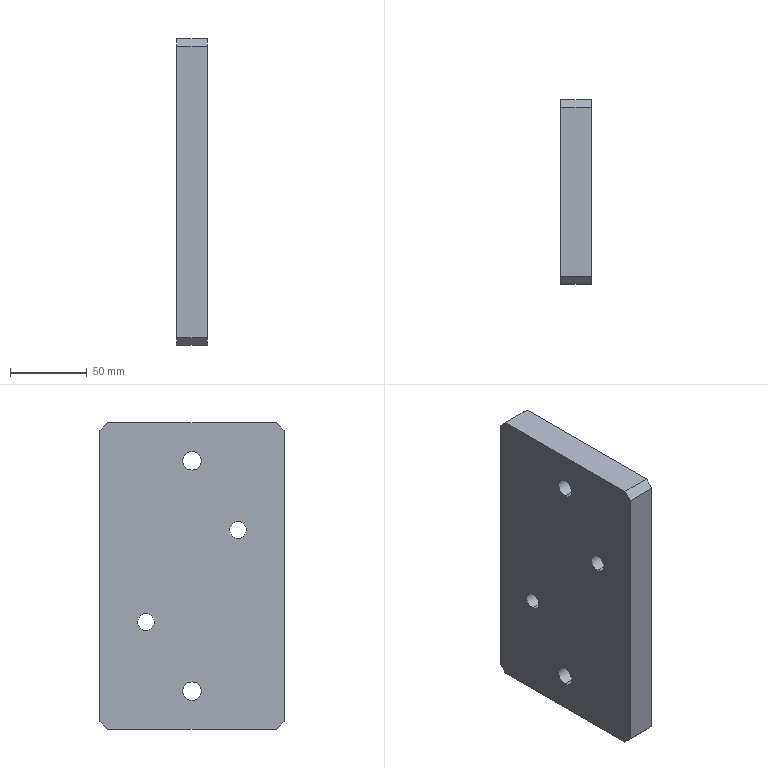Part | SolidWorks | features HoleWzd 2, Chamfer 1, Extrusion 1 | 1 solid | 24 faces | box 20 x 120 x 200 mm | volume 467167 mm3 | cylinder 12 | plane 12 | commonest cylinder face diameters 11 x4 12 x4 18 x4
STEP:
#1=CARTESIAN_POINT('',(0.,0.,81.));
#2=VERTEX_POINT('',#1);
#3=CARTESIAN_POINT('',(0.,0.,69.));
#4=VERTEX_POINT('',#3);
#5=CARTESIAN_POINT('',(0.,0.,75.));
#6=DIRECTION('',(1.,0.,0.));
#7=DIRECTION('',(0.,0.,-1.));
#8=AXIS2_PLACEMENT_3D('',#5,#6,#7);
#9=CIRCLE('',#8,6.);
#10=EDGE_CURVE('',#2,#4,#9,.T.);
#11=ORIENTED_EDGE('',*,*,#10,.F.);
#12=CARTESIAN_POINT('',(20.,0.,81.));
#13=VERTEX_POINT('',#12);
#14=CARTESIAN_POINT('',(20.,0.,81.));
#15=DIRECTION('',(1.,0.,0.));
#16=VECTOR('',#15,1000.);
#17=LINE('',#14,#16);
#18=EDGE_CURVE('',#2,#13,#17,.T.);
#19=ORIENTED_EDGE('',*,*,#18,.T.);
#20=CARTESIAN_POINT('',(20.,0.,69.));
#21=VERTEX_POINT('',#20);
#22=CARTESIAN_POINT('',(20.,0.,75.));
#23=DIRECTION('',(1.,0.,0.));
#24=DIRECTION('',(0.,0.,-1.));
#25=AXIS2_PLACEMENT_3D('',#22,#23,#24);
#26=CIRCLE('',#25,6.);
#27=EDGE_CURVE('',#13,#21,#26,.T.);
#28=ORIENTED_EDGE('',*,*,#27,.T.);
#29=CARTESIAN_POINT('',(20.,0.,69.));
#30=DIRECTION('',(1.,0.,0.));
#31=VECTOR('',#30,1000.);
#32=LINE('',#29,#31);
#33=EDGE_CURVE('',#4,#21,#32,.T.);
#34=ORIENTED_EDGE('',*,*,#33,.F.);
#35=EDGE_LOOP('',(#11,#19,#28,#34));
#36=FACE_OUTER_BOUND('',#35,.T.);
#37=CARTESIAN_POINT('',(20.,0.,75.));
#38=DIRECTION('',(1.,0.,0.));
#39=DIRECTION('',(0.,0.,-1.));
#40=AXIS2_PLACEMENT_3D('',#37,#38,#39);
#41=CYLINDRICAL_SURFACE('',#40,6.);
#42=ADVANCED_FACE('',(#36),#41,.F.);
#43=CARTESIAN_POINT('',(0.,0.,-69.));
#44=VERTEX_POINT('',#43);
#45=CARTESIAN_POINT('',(0.,0.,-81.));
#46=VERTEX_POINT('',#45);
#47=CARTESIAN_POINT('',(0.,0.,-75.));
#48=DIRECTION('',(1.,0.,0.));
#49=DIRECTION('',(0.,0.,-1.));
#50=AXIS2_PLACEMENT_3D('',#47,#48,#49);
#51=CIRCLE('',#50,6.);
#52=EDGE_CURVE('',#44,#46,#51,.T.);
#53=ORIENTED_EDGE('',*,*,#52,.F.);
#54=CARTESIAN_POINT('',(20.,0.,-69.));
#55=VERTEX_POINT('',#54);
#56=CARTESIAN_POINT('',(20.,0.,-69.));
#57=DIRECTION('',(1.,0.,0.));
#58=VECTOR('',#57,1000.);
#59=LINE('',#56,#58);
#60=EDGE_CURVE('',#44,#55,#59,.T.);
#61=ORIENTED_EDGE('',*,*,#60,.T.);
#62=CARTESIAN_POINT('',(20.,0.,-81.));
#63=VERTEX_POINT('',#62);
#64=CARTESIAN_POINT('',(20.,0.,-75.));
#65=DIRECTION('',(1.,0.,0.));
#66=DIRECTION('',(0.,0.,-1.));
#67=AXIS2_PLACEMENT_3D('',#64,#65,#66);
#68=CIRCLE('',#67,6.);
#69=EDGE_CURVE('',#55,#63,#68,.T.);
#70=ORIENTED_EDGE('',*,*,#69,.T.);
#71=CARTESIAN_POINT('',(20.,0.,-81.));
#72=DIRECTION('',(1.,0.,0.));
#73=VECTOR('',#72,1000.);
#74=LINE('',#71,#73);
#75=EDGE_CURVE('',#46,#63,#74,.T.);
#76=ORIENTED_EDGE('',*,*,#75,.F.);
#77=EDGE_LOOP('',(#53,#61,#70,#76));
#78=FACE_OUTER_BOUND('',#77,.T.);
#79=CARTESIAN_POINT('',(20.,0.,-75.));
#80=DIRECTION('',(1.,0.,0.));
#81=DIRECTION('',(0.,0.,-1.));
#82=AXIS2_PLACEMENT_3D('',#79,#80,#81);
#83=CYLINDRICAL_SURFACE('',#82,6.);
#84=ADVANCED_FACE('',(#78),#83,.F.);
#85=CARTESIAN_POINT('',(9.,30.,-21.));
#86=VERTEX_POINT('',#85);
#87=CARTESIAN_POINT('',(9.,30.,-39.));
#88=VERTEX_POINT('',#87);
#89=CARTESIAN_POINT('',(9.,30.,-30.));
#90=DIRECTION('',(1.,0.,0.));
#91=DIRECTION('',(0.,0.,-1.));
#92=AXIS2_PLACEMENT_3D('',#89,#90,#91);
#93=CIRCLE('',#92,9.);
#94=EDGE_CURVE('',#86,#88,#93,.T.);
#95=ORIENTED_EDGE('',*,*,#94,.F.);
#96=CARTESIAN_POINT('',(20.,30.,-21.));
#97=VERTEX_POINT('',#96);
#98=CARTESIAN_POINT('',(20.,30.,-21.));
#99=DIRECTION('',(1.,0.,0.));
#100=VECTOR('',#99,1000.);
#101=LINE('',#98,#100);
#102=EDGE_CURVE('',#86,#97,#101,.T.);
#103=ORIENTED_EDGE('',*,*,#102,.T.);
#104=CARTESIAN_POINT('',(20.,30.,-39.));
#105=VERTEX_POINT('',#104);
#106=CARTESIAN_POINT('',(20.,30.,-30.));
#107=DIRECTION('',(1.,0.,0.));
#108=DIRECTION('',(0.,0.,-1.));
#109=AXIS2_PLACEMENT_3D('',#106,#107,#108);
#110=CIRCLE('',#109,9.);
#111=EDGE_CURVE('',#97,#105,#110,.T.);
#112=ORIENTED_EDGE('',*,*,#111,.T.);
#113=CARTESIAN_POINT('',(20.,30.,-39.));
#114=DIRECTION('',(1.,0.,0.));
#115=VECTOR('',#114,1000.);
#116=LINE('',#113,#115);
#117=EDGE_CURVE('',#88,#105,#116,.T.);
#118=ORIENTED_EDGE('',*,*,#117,.F.);
#119=EDGE_LOOP('',(#95,#103,#112,#118));
#120=FACE_OUTER_BOUND('',#119,.T.);
#121=CARTESIAN_POINT('',(20.,30.,-30.));
#122=DIRECTION('',(1.,0.,0.));
#123=DIRECTION('',(0.,0.,-1.));
#124=AXIS2_PLACEMENT_3D('',#121,#122,#123);
#125=CYLINDRICAL_SURFACE('',#124,9.);
#126=ADVANCED_FACE('',(#120),#125,.F.);
#127=CARTESIAN_POINT('',(0.,30.,-24.5));
#128=VERTEX_POINT('',#127);
#129=CARTESIAN_POINT('',(0.,30.,-35.5));
#130=VERTEX_POINT('',#129);
#131=CARTESIAN_POINT('',(0.,30.,-30.));
#132=DIRECTION('',(1.,0.,0.));
#133=DIRECTION('',(0.,0.,-1.));
#134=AXIS2_PLACEMENT_3D('',#131,#132,#133);
#135=CIRCLE('',#134,5.5);
#136=EDGE_CURVE('',#128,#130,#135,.T.);
#137=ORIENTED_EDGE('',*,*,#136,.F.);
#138=CARTESIAN_POINT('',(9.,30.,-24.5));
#139=VERTEX_POINT('',#138);
#140=CARTESIAN_POINT('',(20.,30.,-24.5));
#141=DIRECTION('',(1.,0.,0.));
#142=VECTOR('',#141,1000.);
#143=LINE('',#140,#142);
#144=EDGE_CURVE('',#128,#139,#143,.T.);
#145=ORIENTED_EDGE('',*,*,#144,.T.);
#146=CARTESIAN_POINT('',(9.,30.,-35.5));
#147=VERTEX_POINT('',#146);
#148=CARTESIAN_POINT('',(9.,30.,-30.));
#149=DIRECTION('',(1.,0.,0.));
#150=DIRECTION('',(0.,0.,-1.));
#151=AXIS2_PLACEMENT_3D('',#148,#149,#150);
#152=CIRCLE('',#151,5.5);
#153=EDGE_CURVE('',#139,#147,#152,.T.);
#154=ORIENTED_EDGE('',*,*,#153,.T.);
#155=CARTESIAN_POINT('',(20.,30.,-35.5));
#156=DIRECTION('',(1.,0.,0.));
#157=VECTOR('',#156,1000.);
#158=LINE('',#155,#157);
#159=EDGE_CURVE('',#130,#147,#158,.T.);
#160=ORIENTED_EDGE('',*,*,#159,.F.);
#161=EDGE_LOOP('',(#137,#145,#154,#160));
#162=FACE_OUTER_BOUND('',#161,.T.);
#163=CARTESIAN_POINT('',(20.,30.,-30.));
#164=DIRECTION('',(1.,0.,0.));
#165=DIRECTION('',(0.,0.,-1.));
#166=AXIS2_PLACEMENT_3D('',#163,#164,#165);
#167=CYLINDRICAL_SURFACE('',#166,5.5);
#168=ADVANCED_FACE('',(#162),#167,.F.);
#169=CARTESIAN_POINT('',(9.,-30.,39.));
#170=VERTEX_POINT('',#169);
#171=CARTESIAN_POINT('',(9.,-30.,21.));
#172=VERTEX_POINT('',#171);
#173=CARTESIAN_POINT('',(9.,-30.,30.));
#174=DIRECTION('',(1.,0.,0.));
#175=DIRECTION('',(0.,0.,-1.));
#176=AXIS2_PLACEMENT_3D('',#173,#174,#175);
#177=CIRCLE('',#176,9.);
#178=EDGE_CURVE('',#170,#172,#177,.T.);
#179=ORIENTED_EDGE('',*,*,#178,.F.);
#180=CARTESIAN_POINT('',(20.,-30.,39.));
#181=VERTEX_POINT('',#180);
#182=CARTESIAN_POINT('',(20.,-30.,39.));
#183=DIRECTION('',(1.,0.,0.));
#184=VECTOR('',#183,1000.);
#185=LINE('',#182,#184);
#186=EDGE_CURVE('',#170,#181,#185,.T.);
#187=ORIENTED_EDGE('',*,*,#186,.T.);
#188=CARTESIAN_POINT('',(20.,-30.,21.));
#189=VERTEX_POINT('',#188);
#190=CARTESIAN_POINT('',(20.,-30.,30.));
#191=DIRECTION('',(1.,0.,0.));
#192=DIRECTION('',(0.,0.,-1.));
#193=AXIS2_PLACEMENT_3D('',#190,#191,#192);
#194=CIRCLE('',#193,9.);
#195=EDGE_CURVE('',#181,#189,#194,.T.);
#196=ORIENTED_EDGE('',*,*,#195,.T.);
#197=CARTESIAN_POINT('',(20.,-30.,21.));
#198=DIRECTION('',(1.,0.,0.));
#199=VECTOR('',#198,1000.);
#200=LINE('',#197,#199);
#201=EDGE_CURVE('',#172,#189,#200,.T.);
#202=ORIENTED_EDGE('',*,*,#201,.F.);
#203=EDGE_LOOP('',(#179,#187,#196,#202));
#204=FACE_OUTER_BOUND('',#203,.T.);
#205=CARTESIAN_POINT('',(20.,-30.,30.));
#206=DIRECTION('',(1.,0.,0.));
#207=DIRECTION('',(0.,0.,-1.));
#208=AXIS2_PLACEMENT_3D('',#205,#206,#207);
#209=CYLINDRICAL_SURFACE('',#208,9.);
#210=ADVANCED_FACE('',(#204),#209,.F.);
#211=CARTESIAN_POINT('',(0.,-30.,35.5));
#212=VERTEX_POINT('',#211);
#213=CARTESIAN_POINT('',(0.,-30.,24.5));
#214=VERTEX_POINT('',#213);
#215=CARTESIAN_POINT('',(0.,-30.,30.));
#216=DIRECTION('',(1.,0.,0.));
#217=DIRECTION('',(0.,0.,-1.));
#218=AXIS2_PLACEMENT_3D('',#215,#216,#217);
#219=CIRCLE('',#218,5.5);
#220=EDGE_CURVE('',#212,#214,#219,.T.);
#221=ORIENTED_EDGE('',*,*,#220,.F.);
#222=CARTESIAN_POINT('',(9.,-30.,35.5));
#223=VERTEX_POINT('',#222);
#224=CARTESIAN_POINT('',(20.,-30.,35.5));
#225=DIRECTION('',(1.,0.,0.));
#226=VECTOR('',#225,1000.);
#227=LINE('',#224,#226);
#228=EDGE_CURVE('',#212,#223,#227,.T.);
#229=ORIENTED_EDGE('',*,*,#228,.T.);
#230=CARTESIAN_POINT('',(9.,-30.,24.5));
#231=VERTEX_POINT('',#230);
#232=CARTESIAN_POINT('',(9.,-30.,30.));
#233=DIRECTION('',(1.,0.,0.));
#234=DIRECTION('',(0.,0.,-1.));
#235=AXIS2_PLACEMENT_3D('',#232,#233,#234);
#236=CIRCLE('',#235,5.5);
#237=EDGE_CURVE('',#223,#231,#236,.T.);
#238=ORIENTED_EDGE('',*,*,#237,.T.);
#239=CARTESIAN_POINT('',(20.,-30.,24.5));
#240=DIRECTION('',(1.,0.,0.));
#241=VECTOR('',#240,1000.);
#242=LINE('',#239,#241);
#243=EDGE_CURVE('',#214,#231,#242,.T.);
#244=ORIENTED_EDGE('',*,*,#243,.F.);
#245=EDGE_LOOP('',(#221,#229,#238,#244));
#246=FACE_OUTER_BOUND('',#245,.T.);
#247=CARTESIAN_POINT('',(20.,-30.,30.));
#248=DIRECTION('',(1.,0.,0.));
#249=DIRECTION('',(0.,0.,-1.));
#250=AXIS2_PLACEMENT_3D('',#247,#248,#249);
#251=CYLINDRICAL_SURFACE('',#250,5.5);
#252=ADVANCED_FACE('',(#246),#251,.F.);
#253=CARTESIAN_POINT('',(0.,-55.,-100.));
#254=VERTEX_POINT('',#253);
#255=CARTESIAN_POINT('',(0.,55.,-100.));
#256=VERTEX_POINT('',#255);
#257=CARTESIAN_POINT('',(0.,60.,-100.));
#258=DIRECTION('',(0.,1.,0.));
#259=VECTOR('',#258,1000.);
#260=LINE('',#257,#259);
#261=EDGE_CURVE('',#254,#256,#260,.T.);
#262=ORIENTED_EDGE('',*,*,#261,.T.);
#263=CARTESIAN_POINT('',(20.,55.,-100.));
#264=VERTEX_POINT('',#263);
#265=CARTESIAN_POINT('',(20.,55.,-100.));
#266=DIRECTION('',(1.,0.,0.));
#267=VECTOR('',#266,1000.);
#268=LINE('',#265,#267);
#269=EDGE_CURVE('',#256,#264,#268,.T.);
#270=ORIENTED_EDGE('',*,*,#269,.T.);
#271=CARTESIAN_POINT('',(20.,-55.,-100.));
#272=VERTEX_POINT('',#271);
#273=CARTESIAN_POINT('',(20.,60.,-100.));
#274=DIRECTION('',(0.,1.,0.));
#275=VECTOR('',#274,1000.);
#276=LINE('',#273,#275);
#277=EDGE_CURVE('',#272,#264,#276,.T.);
#278=ORIENTED_EDGE('',*,*,#277,.F.);
#279=CARTESIAN_POINT('',(20.,-55.,-100.));
#280=DIRECTION('',(-1.,0.,0.));
#281=VECTOR('',#280,1000.);
#282=LINE('',#279,#281);
#283=EDGE_CURVE('',#272,#254,#282,.T.);
#284=ORIENTED_EDGE('',*,*,#283,.T.);
#285=EDGE_LOOP('',(#262,#270,#278,#284));
#286=FACE_OUTER_BOUND('',#285,.T.);
#287=CARTESIAN_POINT('',(20.,60.,-100.));
#288=DIRECTION('',(0.,0.,1.));
#289=DIRECTION('',(0.,-1.,0.));
#290=AXIS2_PLACEMENT_3D('',#287,#288,#289);
#291=PLANE('',#290);
#292=ADVANCED_FACE('',(#286),#291,.F.);
#293=CARTESIAN_POINT('',(0.,60.,-95.));
#294=VERTEX_POINT('',#293);
#295=CARTESIAN_POINT('',(0.,60.,95.));
#296=VERTEX_POINT('',#295);
#297=CARTESIAN_POINT('',(0.,60.,100.));
#298=DIRECTION('',(0.,0.,1.));
#299=VECTOR('',#298,1000.);
#300=LINE('',#297,#299);
#301=EDGE_CURVE('',#294,#296,#300,.T.);
#302=ORIENTED_EDGE('',*,*,#301,.T.);
#303=CARTESIAN_POINT('',(20.,60.,95.));
#304=VERTEX_POINT('',#303);
#305=CARTESIAN_POINT('',(20.,60.,95.));
#306=DIRECTION('',(1.,0.,0.));
#307=VECTOR('',#306,1000.);
#308=LINE('',#305,#307);
#309=EDGE_CURVE('',#296,#304,#308,.T.);
#310=ORIENTED_EDGE('',*,*,#309,.T.);
#311=CARTESIAN_POINT('',(20.,60.,-95.));
#312=VERTEX_POINT('',#311);
#313=CARTESIAN_POINT('',(20.,60.,100.));
#314=DIRECTION('',(0.,0.,1.));
#315=VECTOR('',#314,1000.);
#316=LINE('',#313,#315);
#317=EDGE_CURVE('',#312,#304,#316,.T.);
#318=ORIENTED_EDGE('',*,*,#317,.F.);
#319=CARTESIAN_POINT('',(20.,60.,-95.));
#320=DIRECTION('',(-1.,0.,0.));
#321=VECTOR('',#320,1000.);
#322=LINE('',#319,#321);
#323=EDGE_CURVE('',#312,#294,#322,.T.);
#324=ORIENTED_EDGE('',*,*,#323,.T.);
#325=EDGE_LOOP('',(#302,#310,#318,#324));
#326=FACE_OUTER_BOUND('',#325,.T.);
#327=CARTESIAN_POINT('',(20.,60.,100.));
#328=DIRECTION('',(0.,-1.,0.));
#329=DIRECTION('',(0.,0.,-1.));
#330=AXIS2_PLACEMENT_3D('',#327,#328,#329);
#331=PLANE('',#330);
#332=ADVANCED_FACE('',(#326),#331,.F.);
#333=CARTESIAN_POINT('',(20.,55.,100.));
#334=VERTEX_POINT('',#333);
#335=CARTESIAN_POINT('',(20.,-55.,100.));
#336=VERTEX_POINT('',#335);
#337=CARTESIAN_POINT('',(20.,60.,100.));
#338=DIRECTION('',(0.,-1.,0.));
#339=VECTOR('',#338,1000.);
#340=LINE('',#337,#339);
#341=EDGE_CURVE('',#334,#336,#340,.T.);
#342=ORIENTED_EDGE('',*,*,#341,.F.);
#343=CARTESIAN_POINT('',(0.,55.,100.));
#344=VERTEX_POINT('',#343);
#345=CARTESIAN_POINT('',(20.,55.,100.));
#346=DIRECTION('',(-1.,0.,0.));
#347=VECTOR('',#346,1000.);
#348=LINE('',#345,#347);
#349=EDGE_CURVE('',#334,#344,#348,.T.);
#350=ORIENTED_EDGE('',*,*,#349,.T.);
#351=CARTESIAN_POINT('',(0.,-55.,100.));
#352=VERTEX_POINT('',#351);
#353=CARTESIAN_POINT('',(0.,60.,100.));
#354=DIRECTION('',(0.,-1.,0.));
#355=VECTOR('',#354,1000.);
#356=LINE('',#353,#355);
#357=EDGE_CURVE('',#344,#352,#356,.T.);
#358=ORIENTED_EDGE('',*,*,#357,.T.);
#359=CARTESIAN_POINT('',(20.,-55.,100.));
#360=DIRECTION('',(1.,0.,0.));
#361=VECTOR('',#360,1000.);
#362=LINE('',#359,#361);
#363=EDGE_CURVE('',#352,#336,#362,.T.);
#364=ORIENTED_EDGE('',*,*,#363,.T.);
#365=EDGE_LOOP('',(#342,#350,#358,#364));
#366=FACE_OUTER_BOUND('',#365,.T.);
#367=CARTESIAN_POINT('',(20.,60.,100.));
#368=DIRECTION('',(0.,0.,-1.));
#369=DIRECTION('',(0.,1.,0.));
#370=AXIS2_PLACEMENT_3D('',#367,#368,#369);
#371=PLANE('',#370);
#372=ADVANCED_FACE('',(#366),#371,.F.);
#373=CARTESIAN_POINT('',(0.,-60.,95.));
#374=VERTEX_POINT('',#373);
#375=CARTESIAN_POINT('',(0.,-60.,-95.));
#376=VERTEX_POINT('',#375);
#377=CARTESIAN_POINT('',(0.,-60.,100.));
#378=DIRECTION('',(0.,0.,-1.));
#379=VECTOR('',#378,1000.);
#380=LINE('',#377,#379);
#381=EDGE_CURVE('',#374,#376,#380,.T.);
#382=ORIENTED_EDGE('',*,*,#381,.T.);
#383=CARTESIAN_POINT('',(20.,-60.,-95.));
#384=VERTEX_POINT('',#383);
#385=CARTESIAN_POINT('',(20.,-60.,-95.));
#386=DIRECTION('',(1.,0.,0.));
#387=VECTOR('',#386,1000.);
#388=LINE('',#385,#387);
#389=EDGE_CURVE('',#376,#384,#388,.T.);
#390=ORIENTED_EDGE('',*,*,#389,.T.);
#391=CARTESIAN_POINT('',(20.,-60.,95.));
#392=VERTEX_POINT('',#391);
#393=CARTESIAN_POINT('',(20.,-60.,100.));
#394=DIRECTION('',(0.,0.,-1.));
#395=VECTOR('',#394,1000.);
#396=LINE('',#393,#395);
#397=EDGE_CURVE('',#392,#384,#396,.T.);
#398=ORIENTED_EDGE('',*,*,#397,.F.);
#399=CARTESIAN_POINT('',(20.,-60.,95.));
#400=DIRECTION('',(-1.,0.,0.));
#401=VECTOR('',#400,1000.);
#402=LINE('',#399,#401);
#403=EDGE_CURVE('',#392,#374,#402,.T.);
#404=ORIENTED_EDGE('',*,*,#403,.T.);
#405=EDGE_LOOP('',(#382,#390,#398,#404));
#406=FACE_OUTER_BOUND('',#405,.T.);
#407=CARTESIAN_POINT('',(20.,-60.,100.));
#408=DIRECTION('',(0.,1.,0.));
#409=DIRECTION('',(0.,0.,1.));
#410=AXIS2_PLACEMENT_3D('',#407,#408,#409);
#411=PLANE('',#410);
#412=ADVANCED_FACE('',(#406),#411,.F.);
#413=CARTESIAN_POINT('',(20.,0.,75.));
#414=DIRECTION('',(1.,0.,0.));
#415=DIRECTION('',(0.,0.,-1.));
#416=AXIS2_PLACEMENT_3D('',#413,#414,#415);
#417=CIRCLE('',#416,6.);
#418=EDGE_CURVE('',#21,#13,#417,.T.);
#419=ORIENTED_EDGE('',*,*,#418,.F.);
#420=ORIENTED_EDGE('',*,*,#27,.F.);
#421=EDGE_LOOP('',(#419,#420));
#422=FACE_BOUND('',#421,.T.);
#423=CARTESIAN_POINT('',(20.,0.,-75.));
#424=DIRECTION('',(1.,0.,0.));
#425=DIRECTION('',(0.,0.,-1.));
#426=AXIS2_PLACEMENT_3D('',#423,#424,#425);
#427=CIRCLE('',#426,6.);
#428=EDGE_CURVE('',#63,#55,#427,.T.);
#429=ORIENTED_EDGE('',*,*,#428,.F.);
#430=ORIENTED_EDGE('',*,*,#69,.F.);
#431=EDGE_LOOP('',(#429,#430));
#432=FACE_BOUND('',#431,.T.);
#433=CARTESIAN_POINT('',(20.,30.,-30.));
#434=DIRECTION('',(1.,0.,0.));
#435=DIRECTION('',(0.,0.,-1.));
#436=AXIS2_PLACEMENT_3D('',#433,#434,#435);
#437=CIRCLE('',#436,9.);
#438=EDGE_CURVE('',#105,#97,#437,.T.);
#439=ORIENTED_EDGE('',*,*,#438,.F.);
#440=ORIENTED_EDGE('',*,*,#111,.F.);
#441=EDGE_LOOP('',(#439,#440));
#442=FACE_BOUND('',#441,.T.);
#443=CARTESIAN_POINT('',(20.,-30.,30.));
#444=DIRECTION('',(1.,0.,0.));
#445=DIRECTION('',(0.,0.,-1.));
#446=AXIS2_PLACEMENT_3D('',#443,#444,#445);
#447=CIRCLE('',#446,9.);
#448=EDGE_CURVE('',#189,#181,#447,.T.);
#449=ORIENTED_EDGE('',*,*,#448,.F.);
#450=ORIENTED_EDGE('',*,*,#195,.F.);
#451=EDGE_LOOP('',(#449,#450));
#452=FACE_BOUND('',#451,.T.);
#453=ORIENTED_EDGE('',*,*,#317,.T.);
#454=CARTESIAN_POINT('',(20.,77.5,77.5));
#455=DIRECTION('',(0.,-0.7071,0.7071));
#456=VECTOR('',#455,1000.);
#457=LINE('',#454,#456);
#458=EDGE_CURVE('',#304,#334,#457,.T.);
#459=ORIENTED_EDGE('',*,*,#458,.T.);
#460=ORIENTED_EDGE('',*,*,#341,.T.);
#461=CARTESIAN_POINT('',(20.,-77.5,77.5));
#462=DIRECTION('',(0.,-0.7071,-0.7071));
#463=VECTOR('',#462,1000.);
#464=LINE('',#461,#463);
#465=EDGE_CURVE('',#336,#392,#464,.T.);
#466=ORIENTED_EDGE('',*,*,#465,.T.);
#467=ORIENTED_EDGE('',*,*,#397,.T.);
#468=CARTESIAN_POINT('',(20.,-77.5,-77.5));
#469=DIRECTION('',(0.,0.7071,-0.7071));
#470=VECTOR('',#469,1000.);
#471=LINE('',#468,#470);
#472=EDGE_CURVE('',#384,#272,#471,.T.);
#473=ORIENTED_EDGE('',*,*,#472,.T.);
#474=ORIENTED_EDGE('',*,*,#277,.T.);
#475=CARTESIAN_POINT('',(20.,77.5,-77.5));
#476=DIRECTION('',(0.,0.7071,0.7071));
#477=VECTOR('',#476,1000.);
#478=LINE('',#475,#477);
#479=EDGE_CURVE('',#264,#312,#478,.T.);
#480=ORIENTED_EDGE('',*,*,#479,.T.);
#481=EDGE_LOOP('',(#453,#459,#460,#466,#467,#473,#474,#480));
#482=FACE_OUTER_BOUND('',#481,.T.);
#483=CARTESIAN_POINT('',(20.,0.,0.));
#484=DIRECTION('',(1.,0.,0.));
#485=DIRECTION('',(0.,0.,-1.));
#486=AXIS2_PLACEMENT_3D('',#483,#484,#485);
#487=PLANE('',#486);
#488=ADVANCED_FACE('',(#422,#432,#442,#452,#482),#487,.T.);
#489=CARTESIAN_POINT('',(0.,0.,75.));
#490=DIRECTION('',(1.,0.,0.));
#491=DIRECTION('',(0.,0.,-1.));
#492=AXIS2_PLACEMENT_3D('',#489,#490,#491);
#493=CIRCLE('',#492,6.);
#494=EDGE_CURVE('',#4,#2,#493,.T.);
#495=ORIENTED_EDGE('',*,*,#494,.T.);
#496=ORIENTED_EDGE('',*,*,#10,.T.);
#497=EDGE_LOOP('',(#495,#496));
#498=FACE_BOUND('',#497,.T.);
#499=CARTESIAN_POINT('',(0.,0.,-75.));
#500=DIRECTION('',(1.,0.,0.));
#501=DIRECTION('',(0.,0.,-1.));
#502=AXIS2_PLACEMENT_3D('',#499,#500,#501);
#503=CIRCLE('',#502,6.);
#504=EDGE_CURVE('',#46,#44,#503,.T.);
#505=ORIENTED_EDGE('',*,*,#504,.T.);
#506=ORIENTED_EDGE('',*,*,#52,.T.);
#507=EDGE_LOOP('',(#505,#506));
#508=FACE_BOUND('',#507,.T.);
#509=CARTESIAN_POINT('',(0.,30.,-30.));
#510=DIRECTION('',(1.,0.,0.));
#511=DIRECTION('',(0.,0.,-1.));
#512=AXIS2_PLACEMENT_3D('',#509,#510,#511);
#513=CIRCLE('',#512,5.5);
#514=EDGE_CURVE('',#130,#128,#513,.T.);
#515=ORIENTED_EDGE('',*,*,#514,.T.);
#516=ORIENTED_EDGE('',*,*,#136,.T.);
#517=EDGE_LOOP('',(#515,#516));
#518=FACE_BOUND('',#517,.T.);
#519=CARTESIAN_POINT('',(0.,-30.,30.));
#520=DIRECTION('',(1.,0.,0.));
#521=DIRECTION('',(0.,0.,-1.));
#522=AXIS2_PLACEMENT_3D('',#519,#520,#521);
#523=CIRCLE('',#522,5.5);
#524=EDGE_CURVE('',#214,#212,#523,.T.);
#525=ORIENTED_EDGE('',*,*,#524,.T.);
#526=ORIENTED_EDGE('',*,*,#220,.T.);
#527=EDGE_LOOP('',(#525,#526));
#528=FACE_BOUND('',#527,.T.);
#529=ORIENTED_EDGE('',*,*,#357,.F.);
#530=CARTESIAN_POINT('',(0.,55.,100.));
#531=DIRECTION('',(0.,0.7071,-0.7071));
#532=VECTOR('',#531,1000.);
#533=LINE('',#530,#532);
#534=EDGE_CURVE('',#344,#296,#533,.T.);
#535=ORIENTED_EDGE('',*,*,#534,.T.);
#536=ORIENTED_EDGE('',*,*,#301,.F.);
#537=CARTESIAN_POINT('',(0.,60.,-95.));
#538=DIRECTION('',(0.,-0.7071,-0.7071));
#539=VECTOR('',#538,1000.);
#540=LINE('',#537,#539);
#541=EDGE_CURVE('',#294,#256,#540,.T.);
#542=ORIENTED_EDGE('',*,*,#541,.T.);
#543=ORIENTED_EDGE('',*,*,#261,.F.);
#544=CARTESIAN_POINT('',(0.,-55.,-100.));
#545=DIRECTION('',(0.,-0.7071,0.7071));
#546=VECTOR('',#545,1000.);
#547=LINE('',#544,#546);
#548=EDGE_CURVE('',#254,#376,#547,.T.);
#549=ORIENTED_EDGE('',*,*,#548,.T.);
#550=ORIENTED_EDGE('',*,*,#381,.F.);
#551=CARTESIAN_POINT('',(0.,-60.,95.));
#552=DIRECTION('',(0.,0.7071,0.7071));
#553=VECTOR('',#552,1000.);
#554=LINE('',#551,#553);
#555=EDGE_CURVE('',#374,#352,#554,.T.);
#556=ORIENTED_EDGE('',*,*,#555,.T.);
#557=EDGE_LOOP('',(#529,#535,#536,#542,#543,#549,#550,#556));
#558=FACE_OUTER_BOUND('',#557,.T.);
#559=CARTESIAN_POINT('',(0.,0.,0.));
#560=DIRECTION('',(1.,0.,0.));
#561=DIRECTION('',(0.,0.,-1.));
#562=AXIS2_PLACEMENT_3D('',#559,#560,#561);
#563=PLANE('',#562);
#564=ADVANCED_FACE('',(#498,#508,#518,#528,#558),#563,.F.);
#565=ORIENTED_EDGE('',*,*,#228,.F.);
#566=ORIENTED_EDGE('',*,*,#524,.F.);
#567=ORIENTED_EDGE('',*,*,#243,.T.);
#568=CARTESIAN_POINT('',(9.,-30.,30.));
#569=DIRECTION('',(1.,0.,0.));
#570=DIRECTION('',(0.,0.,-1.));
#571=AXIS2_PLACEMENT_3D('',#568,#569,#570);
#572=CIRCLE('',#571,5.5);
#573=EDGE_CURVE('',#231,#223,#572,.T.);
#574=ORIENTED_EDGE('',*,*,#573,.T.);
#575=EDGE_LOOP('',(#565,#566,#567,#574));
#576=FACE_OUTER_BOUND('',#575,.T.);
#577=CARTESIAN_POINT('',(20.,-30.,30.));
#578=DIRECTION('',(1.,0.,0.));
#579=DIRECTION('',(0.,0.,-1.));
#580=AXIS2_PLACEMENT_3D('',#577,#578,#579);
#581=CYLINDRICAL_SURFACE('',#580,5.5);
#582=ADVANCED_FACE('',(#576),#581,.F.);
#583=ORIENTED_EDGE('',*,*,#573,.F.);
#584=ORIENTED_EDGE('',*,*,#237,.F.);
#585=EDGE_LOOP('',(#583,#584));
#586=FACE_BOUND('',#585,.T.);
#587=CARTESIAN_POINT('',(9.,-30.,30.));
#588=DIRECTION('',(1.,0.,0.));
#589=DIRECTION('',(0.,0.,-1.));
#590=AXIS2_PLACEMENT_3D('',#587,#588,#589);
#591=CIRCLE('',#590,9.);
#592=EDGE_CURVE('',#172,#170,#591,.T.);
#593=ORIENTED_EDGE('',*,*,#592,.T.);
#594=ORIENTED_EDGE('',*,*,#178,.T.);
#595=EDGE_LOOP('',(#593,#594));
#596=FACE_OUTER_BOUND('',#595,.T.);
#597=CARTESIAN_POINT('',(9.,-24.5,30.));
#598=DIRECTION('',(-1.,0.,0.));
#599=DIRECTION('',(0.,0.,1.));
#600=AXIS2_PLACEMENT_3D('',#597,#598,#599);
#601=PLANE('',#600);
#602=ADVANCED_FACE('',(#586,#596),#601,.F.);
#603=ORIENTED_EDGE('',*,*,#186,.F.);
#604=ORIENTED_EDGE('',*,*,#592,.F.);
#605=ORIENTED_EDGE('',*,*,#201,.T.);
#606=ORIENTED_EDGE('',*,*,#448,.T.);
#607=EDGE_LOOP('',(#603,#604,#605,#606));
#608=FACE_OUTER_BOUND('',#607,.T.);
#609=CARTESIAN_POINT('',(20.,-30.,30.));
#610=DIRECTION('',(1.,0.,0.));
#611=DIRECTION('',(0.,0.,-1.));
#612=AXIS2_PLACEMENT_3D('',#609,#610,#611);
#613=CYLINDRICAL_SURFACE('',#612,9.);
#614=ADVANCED_FACE('',(#608),#613,.F.);
#615=ORIENTED_EDGE('',*,*,#144,.F.);
#616=ORIENTED_EDGE('',*,*,#514,.F.);
#617=ORIENTED_EDGE('',*,*,#159,.T.);
#618=CARTESIAN_POINT('',(9.,30.,-30.));
#619=DIRECTION('',(1.,0.,0.));
#620=DIRECTION('',(0.,0.,-1.));
#621=AXIS2_PLACEMENT_3D('',#618,#619,#620);
#622=CIRCLE('',#621,5.5);
#623=EDGE_CURVE('',#147,#139,#622,.T.);
#624=ORIENTED_EDGE('',*,*,#623,.T.);
#625=EDGE_LOOP('',(#615,#616,#617,#624));
#626=FACE_OUTER_BOUND('',#625,.T.);
#627=CARTESIAN_POINT('',(20.,30.,-30.));
#628=DIRECTION('',(1.,0.,0.));
#629=DIRECTION('',(0.,0.,-1.));
#630=AXIS2_PLACEMENT_3D('',#627,#628,#629);
#631=CYLINDRICAL_SURFACE('',#630,5.5);
#632=ADVANCED_FACE('',(#626),#631,.F.);
#633=ORIENTED_EDGE('',*,*,#623,.F.);
#634=ORIENTED_EDGE('',*,*,#153,.F.);
#635=EDGE_LOOP('',(#633,#634));
#636=FACE_BOUND('',#635,.T.);
#637=CARTESIAN_POINT('',(9.,30.,-30.));
#638=DIRECTION('',(1.,0.,0.));
#639=DIRECTION('',(0.,0.,-1.));
#640=AXIS2_PLACEMENT_3D('',#637,#638,#639);
#641=CIRCLE('',#640,9.);
#642=EDGE_CURVE('',#88,#86,#641,.T.);
#643=ORIENTED_EDGE('',*,*,#642,.T.);
#644=ORIENTED_EDGE('',*,*,#94,.T.);
#645=EDGE_LOOP('',(#643,#644));
#646=FACE_OUTER_BOUND('',#645,.T.);
#647=CARTESIAN_POINT('',(9.,35.5,-30.));
#648=DIRECTION('',(-1.,0.,0.));
#649=DIRECTION('',(0.,0.,1.));
#650=AXIS2_PLACEMENT_3D('',#647,#648,#649);
#651=PLANE('',#650);
#652=ADVANCED_FACE('',(#636,#646),#651,.F.);
#653=ORIENTED_EDGE('',*,*,#102,.F.);
#654=ORIENTED_EDGE('',*,*,#642,.F.);
#655=ORIENTED_EDGE('',*,*,#117,.T.);
#656=ORIENTED_EDGE('',*,*,#438,.T.);
#657=EDGE_LOOP('',(#653,#654,#655,#656));
#658=FACE_OUTER_BOUND('',#657,.T.);
#659=CARTESIAN_POINT('',(20.,30.,-30.));
#660=DIRECTION('',(1.,0.,0.));
#661=DIRECTION('',(0.,0.,-1.));
#662=AXIS2_PLACEMENT_3D('',#659,#660,#661);
#663=CYLINDRICAL_SURFACE('',#662,9.);
#664=ADVANCED_FACE('',(#658),#663,.F.);
#665=ORIENTED_EDGE('',*,*,#60,.F.);
#666=ORIENTED_EDGE('',*,*,#504,.F.);
#667=ORIENTED_EDGE('',*,*,#75,.T.);
#668=ORIENTED_EDGE('',*,*,#428,.T.);
#669=EDGE_LOOP('',(#665,#666,#667,#668));
#670=FACE_OUTER_BOUND('',#669,.T.);
#671=CARTESIAN_POINT('',(20.,0.,-75.));
#672=DIRECTION('',(1.,0.,0.));
#673=DIRECTION('',(0.,0.,-1.));
#674=AXIS2_PLACEMENT_3D('',#671,#672,#673);
#675=CYLINDRICAL_SURFACE('',#674,6.);
#676=ADVANCED_FACE('',(#670),#675,.F.);
#677=ORIENTED_EDGE('',*,*,#18,.F.);
#678=ORIENTED_EDGE('',*,*,#494,.F.);
#679=ORIENTED_EDGE('',*,*,#33,.T.);
#680=ORIENTED_EDGE('',*,*,#418,.T.);
#681=EDGE_LOOP('',(#677,#678,#679,#680));
#682=FACE_OUTER_BOUND('',#681,.T.);
#683=CARTESIAN_POINT('',(20.,0.,75.));
#684=DIRECTION('',(1.,0.,0.));
#685=DIRECTION('',(0.,0.,-1.));
#686=AXIS2_PLACEMENT_3D('',#683,#684,#685);
#687=CYLINDRICAL_SURFACE('',#686,6.);
#688=ADVANCED_FACE('',(#682),#687,.F.);
#689=ORIENTED_EDGE('',*,*,#458,.F.);
#690=ORIENTED_EDGE('',*,*,#309,.F.);
#691=ORIENTED_EDGE('',*,*,#534,.F.);
#692=ORIENTED_EDGE('',*,*,#349,.F.);
#693=EDGE_LOOP('',(#689,#690,#691,#692));
#694=FACE_OUTER_BOUND('',#693,.T.);
#695=CARTESIAN_POINT('',(20.,55.,100.));
#696=DIRECTION('',(0.,-0.7071,-0.7071));
#697=DIRECTION('',(-1.,0.,0.));
#698=AXIS2_PLACEMENT_3D('',#695,#696,#697);
#699=PLANE('',#698);
#700=ADVANCED_FACE('',(#694),#699,.F.);
#701=ORIENTED_EDGE('',*,*,#479,.F.);
#702=ORIENTED_EDGE('',*,*,#269,.F.);
#703=ORIENTED_EDGE('',*,*,#541,.F.);
#704=ORIENTED_EDGE('',*,*,#323,.F.);
#705=EDGE_LOOP('',(#701,#702,#703,#704));
#706=FACE_OUTER_BOUND('',#705,.T.);
#707=CARTESIAN_POINT('',(20.,60.,-95.));
#708=DIRECTION('',(0.,-0.7071,0.7071));
#709=DIRECTION('',(-1.,0.,0.));
#710=AXIS2_PLACEMENT_3D('',#707,#708,#709);
#711=PLANE('',#710);
#712=ADVANCED_FACE('',(#706),#711,.F.);
#713=ORIENTED_EDGE('',*,*,#472,.F.);
#714=ORIENTED_EDGE('',*,*,#389,.F.);
#715=ORIENTED_EDGE('',*,*,#548,.F.);
#716=ORIENTED_EDGE('',*,*,#283,.F.);
#717=EDGE_LOOP('',(#713,#714,#715,#716));
#718=FACE_OUTER_BOUND('',#717,.T.);
#719=CARTESIAN_POINT('',(20.,-55.,-100.));
#720=DIRECTION('',(0.,0.7071,0.7071));
#721=DIRECTION('',(-1.,0.,0.));
#722=AXIS2_PLACEMENT_3D('',#719,#720,#721);
#723=PLANE('',#722);
#724=ADVANCED_FACE('',(#718),#723,.F.);
#725=ORIENTED_EDGE('',*,*,#465,.F.);
#726=ORIENTED_EDGE('',*,*,#363,.F.);
#727=ORIENTED_EDGE('',*,*,#555,.F.);
#728=ORIENTED_EDGE('',*,*,#403,.F.);
#729=EDGE_LOOP('',(#725,#726,#727,#728));
#730=FACE_OUTER_BOUND('',#729,.T.);
#731=CARTESIAN_POINT('',(20.,-60.,95.));
#732=DIRECTION('',(0.,0.7071,-0.7071));
#733=DIRECTION('',(-1.,0.,0.));
#734=AXIS2_PLACEMENT_3D('',#731,#732,#733);
#735=PLANE('',#734);
#736=ADVANCED_FACE('',(#730),#735,.F.);
#737=CLOSED_SHELL('',(#42,#84,#126,#168,#210,#252,#292,#332,#372,#412,#488,#564,#582,#602,#614,#632,#652,#664,#676,#688,#700,#712,#724,#736));
#738=MANIFOLD_SOLID_BREP('',#737);
#739=CARTESIAN_POINT('',(0.,0.,0.));
#740=DIRECTION('',(0.,0.,1.));
#741=DIRECTION('',(1.,0.,0.));
#742=AXIS2_PLACEMENT_3D('',#739,#740,#741);
#743=(LENGTH_UNIT()NAMED_UNIT(*)SI_UNIT(.MILLI.,.METRE.));
#744=UNCERTAINTY_MEASURE_WITH_UNIT(LENGTH_MEASURE(0.00001),#743,'','');
#745=(NAMED_UNIT(*)PLANE_ANGLE_UNIT()SI_UNIT($,.RADIAN.));
#746=(NAMED_UNIT(*)SI_UNIT($,.STERADIAN.)SOLID_ANGLE_UNIT());
#747=(GEOMETRIC_REPRESENTATION_CONTEXT(3)GLOBAL_UNCERTAINTY_ASSIGNED_CONTEXT((#744))GLOBAL_UNIT_ASSIGNED_CONTEXT((#743,#745,#746))REPRESENTATION_CONTEXT('',''));
#748=ADVANCED_BREP_SHAPE_REPRESENTATION('',(#738,#742),#747);